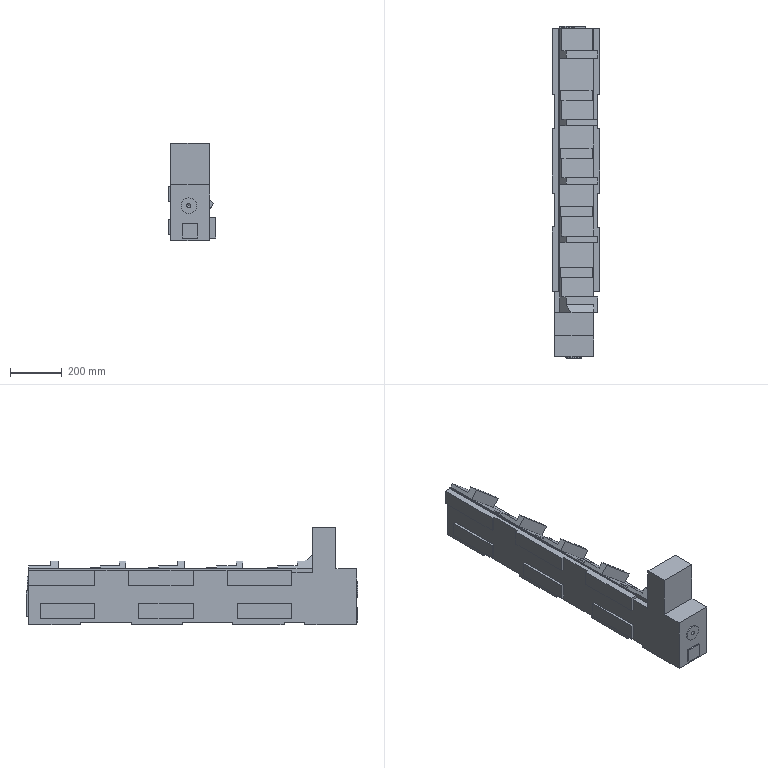Part | NX | features solid 2 | 1 solid | 129 faces | box 185 x 1280 x 375 mm | volume 38220034 mm3 | plane 122 | cylinder 5 | cone 2 | commonest cylinder face diameters 16 x2 50 x1 60 x1 78 x1